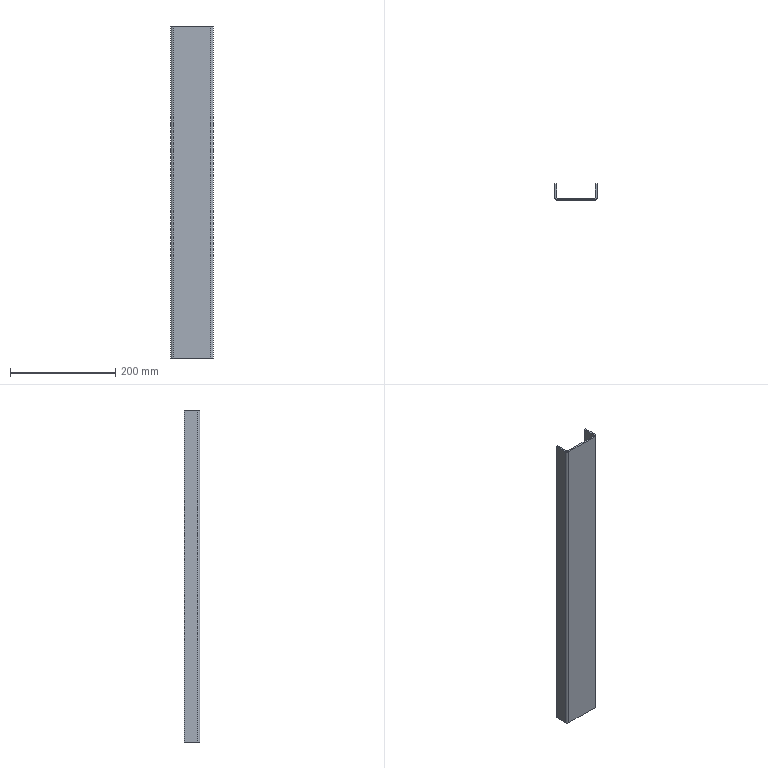Part | STEP file | 1 solid | 22 faces | box 80 x 30 x 630 mm | volume 248393 mm3 | plane 18 | cylinder 4 | commonest cylinder face diameters 3 x2 9 x2
STEP:
#1=CARTESIAN_POINT('',(0.,0.,0.));
#2=DIRECTION('',(0.,0.,1.));
#3=DIRECTION('',(1.,0.,0.));
#4=AXIS2_PLACEMENT_3D('',#1,#2,#3);
#5=CARTESIAN_POINT('',(35.5,-6.24,630.));
#6=VERTEX_POINT('',#5);
#7=CARTESIAN_POINT('',(35.5,-3.24,630.));
#8=VERTEX_POINT('',#7);
#9=CARTESIAN_POINT('',(35.5,-6.24,630.));
#10=DIRECTION('',(0.,1.,0.));
#11=VECTOR('',#10,1.);
#12=LINE('',#9,#11);
#13=CARTESIAN_POINT('',(35.5,-6.24,630.));
#14=DIRECTION('',(0.,0.,1.));
#15=DIRECTION('',(1.,0.,0.));
#16=AXIS2_PLACEMENT_3D('',#13,#14,#15);
#17=PLANE('',#16);
#18=CARTESIAN_POINT('',(0.,0.));
#19=DIRECTION('',(0.,1.));
#20=VECTOR('',#19,1.);
#21=LINE('',#18,#20);
#22=(GEOMETRIC_REPRESENTATION_CONTEXT(2)PARAMETRIC_REPRESENTATION_CONTEXT()REPRESENTATION_CONTEXT('',''));
#23=DEFINITIONAL_REPRESENTATION('',(#21),#22);
#24=PCURVE('',#17,#23);
#25=CARTESIAN_POINT('',(37.,-1.74,630.));
#26=DIRECTION('',(0.,0.,1.));
#27=DIRECTION('',(1.,0.,0.));
#28=AXIS2_PLACEMENT_3D('',#25,#26,#27);
#29=PLANE('',#28);
#30=CARTESIAN_POINT('',(-1.5,-4.5));
#31=DIRECTION('',(0.,1.));
#32=VECTOR('',#31,1.);
#33=LINE('',#30,#32);
#34=(GEOMETRIC_REPRESENTATION_CONTEXT(2)PARAMETRIC_REPRESENTATION_CONTEXT()REPRESENTATION_CONTEXT('',''));
#35=DEFINITIONAL_REPRESENTATION('',(#33),#34);
#36=PCURVE('',#29,#35);
#37=SURFACE_CURVE('',#12,(#24,#36),.PCURVE_S1.);
#38=EDGE_CURVE('',#6,#8,#37,.T.);
#39=ORIENTED_EDGE('',*,*,#38,.F.);
#40=CARTESIAN_POINT('',(40.,-1.74,630.));
#41=VERTEX_POINT('',#40);
#42=CARTESIAN_POINT('',(35.5,-1.74,630.));
#43=DIRECTION('',(0.,0.,-1.));
#44=DIRECTION('',(1.,0.,0.));
#45=AXIS2_PLACEMENT_3D('',#42,#43,#44);
#46=CIRCLE('',#45,4.5);
#47=CARTESIAN_POINT('',(4.5,4.5));
#48=CARTESIAN_POINT('',(4.5,-3.294));
#49=CARTESIAN_POINT('',(-2.25,0.6029));
#50=CARTESIAN_POINT('',(-9.,4.5));
#51=CARTESIAN_POINT('',(-2.25,8.397));
#52=CARTESIAN_POINT('',(4.5,12.294));
#53=CARTESIAN_POINT('',(4.5,4.5));
#54=(BOUNDED_CURVE()B_SPLINE_CURVE(2,(#47,#48,#49,#50,#51,#52,#53),.UNSPECIFIED.,.T.,.F.)B_SPLINE_CURVE_WITH_KNOTS((1,2,2,2,2,1),(-2.094,0.,2.094,4.189,6.283,8.378),.UNSPECIFIED.)CURVE()GEOMETRIC_REPRESENTATION_ITEM()RATIONAL_B_SPLINE_CURVE((1.,0.5,1.,0.5,1.,0.5,1.))REPRESENTATION_ITEM(''));
#55=(GEOMETRIC_REPRESENTATION_CONTEXT(2)PARAMETRIC_REPRESENTATION_CONTEXT()REPRESENTATION_CONTEXT('',''));
#56=DEFINITIONAL_REPRESENTATION('',(#54),#55);
#57=PCURVE('',#17,#56);
#58=CARTESIAN_POINT('',(35.5,-1.74,630.));
#59=DIRECTION('',(0.,0.,-1.));
#60=DIRECTION('',(-1.,0.,0.));
#61=AXIS2_PLACEMENT_3D('',#58,#59,#60);
#62=CYLINDRICAL_SURFACE('',#61,4.5);
#63=CARTESIAN_POINT('',(3.142,0.));
#64=DIRECTION('',(1.,0.));
#65=VECTOR('',#64,1.);
#66=LINE('',#63,#65);
#67=(GEOMETRIC_REPRESENTATION_CONTEXT(2)PARAMETRIC_REPRESENTATION_CONTEXT()REPRESENTATION_CONTEXT('',''));
#68=DEFINITIONAL_REPRESENTATION('',(#66),#67);
#69=PCURVE('',#62,#68);
#70=SURFACE_CURVE('',#46,(#57,#69),.PCURVE_S1.);
#71=EDGE_CURVE('',#41,#6,#70,.T.);
#72=ORIENTED_EDGE('',*,*,#71,.F.);
#73=CARTESIAN_POINT('',(37.,-1.74,630.));
#74=VERTEX_POINT('',#73);
#75=CARTESIAN_POINT('',(37.,-1.74,630.));
#76=DIRECTION('',(1.,0.,0.));
#77=VECTOR('',#76,1.);
#78=LINE('',#75,#77);
#79=CARTESIAN_POINT('',(1.5,4.5));
#80=DIRECTION('',(1.,0.));
#81=VECTOR('',#80,1.);
#82=LINE('',#79,#81);
#83=(GEOMETRIC_REPRESENTATION_CONTEXT(2)PARAMETRIC_REPRESENTATION_CONTEXT()REPRESENTATION_CONTEXT('',''));
#84=DEFINITIONAL_REPRESENTATION('',(#82),#83);
#85=PCURVE('',#17,#84);
#86=CARTESIAN_POINT('',(-35.5,-1.74,630.));
#87=DIRECTION('',(0.,0.,1.));
#88=DIRECTION('',(1.,0.,0.));
#89=AXIS2_PLACEMENT_3D('',#86,#87,#88);
#90=PLANE('',#89);
#91=CARTESIAN_POINT('',(72.5,0.));
#92=DIRECTION('',(1.,0.));
#93=VECTOR('',#92,1.);
#94=LINE('',#91,#93);
#95=(GEOMETRIC_REPRESENTATION_CONTEXT(2)PARAMETRIC_REPRESENTATION_CONTEXT()REPRESENTATION_CONTEXT('',''));
#96=DEFINITIONAL_REPRESENTATION('',(#94),#95);
#97=PCURVE('',#90,#96);
#98=SURFACE_CURVE('',#78,(#85,#97),.PCURVE_S1.);
#99=EDGE_CURVE('',#74,#41,#98,.T.);
#100=ORIENTED_EDGE('',*,*,#99,.F.);
#101=CARTESIAN_POINT('',(35.5,-1.74,630.));
#102=DIRECTION('',(0.,0.,-1.));
#103=DIRECTION('',(1.,0.,0.));
#104=AXIS2_PLACEMENT_3D('',#101,#102,#103);
#105=CIRCLE('',#104,1.5);
#106=CARTESIAN_POINT('',(1.5,4.5));
#107=CARTESIAN_POINT('',(1.5,1.902));
#108=CARTESIAN_POINT('',(-0.75,3.201));
#109=CARTESIAN_POINT('',(-3.,4.5));
#110=CARTESIAN_POINT('',(-0.75,5.799));
#111=CARTESIAN_POINT('',(1.5,7.098));
#112=CARTESIAN_POINT('',(1.5,4.5));
#113=(BOUNDED_CURVE()B_SPLINE_CURVE(2,(#106,#107,#108,#109,#110,#111,#112),.UNSPECIFIED.,.T.,.F.)B_SPLINE_CURVE_WITH_KNOTS((1,2,2,2,2,1),(-2.094,0.,2.094,4.189,6.283,8.378),.UNSPECIFIED.)CURVE()GEOMETRIC_REPRESENTATION_ITEM()RATIONAL_B_SPLINE_CURVE((1.,0.5,1.,0.5,1.,0.5,1.))REPRESENTATION_ITEM(''));
#114=(GEOMETRIC_REPRESENTATION_CONTEXT(2)PARAMETRIC_REPRESENTATION_CONTEXT()REPRESENTATION_CONTEXT('',''));
#115=DEFINITIONAL_REPRESENTATION('',(#113),#114);
#116=PCURVE('',#17,#115);
#117=CARTESIAN_POINT('',(35.5,-1.74,630.));
#118=DIRECTION('',(0.,0.,-1.));
#119=DIRECTION('',(-1.,0.,0.));
#120=AXIS2_PLACEMENT_3D('',#117,#118,#119);
#121=CYLINDRICAL_SURFACE('',#120,1.5);
#122=CARTESIAN_POINT('',(3.142,0.));
#123=DIRECTION('',(1.,0.));
#124=VECTOR('',#123,1.);
#125=LINE('',#122,#124);
#126=(GEOMETRIC_REPRESENTATION_CONTEXT(2)PARAMETRIC_REPRESENTATION_CONTEXT()REPRESENTATION_CONTEXT('',''));
#127=DEFINITIONAL_REPRESENTATION('',(#125),#126);
#128=PCURVE('',#121,#127);
#129=SURFACE_CURVE('',#105,(#116,#128),.PCURVE_S1.);
#130=EDGE_CURVE('',#74,#8,#129,.T.);
#131=ORIENTED_EDGE('',*,*,#130,.T.);
#132=EDGE_LOOP('',(#39,#72,#100,#131));
#133=FACE_BOUND('',#132,.T.);
#134=ADVANCED_FACE('',(#133),#17,.T.);
#135=CARTESIAN_POINT('',(-35.5,-6.24,630.));
#136=VERTEX_POINT('',#135);
#137=CARTESIAN_POINT('',(-40.,-6.24,630.));
#138=DIRECTION('',(-1.,0.,0.));
#139=VECTOR('',#138,1.);
#140=LINE('',#137,#139);
#141=CARTESIAN_POINT('',(-77.,-4.5));
#142=DIRECTION('',(-1.,0.));
#143=VECTOR('',#142,1.);
#144=LINE('',#141,#143);
#145=(GEOMETRIC_REPRESENTATION_CONTEXT(2)PARAMETRIC_REPRESENTATION_CONTEXT()REPRESENTATION_CONTEXT('',''));
#146=DEFINITIONAL_REPRESENTATION('',(#144),#145);
#147=PCURVE('',#29,#146);
#148=CARTESIAN_POINT('',(-40.,-6.24,630.));
#149=DIRECTION('',(0.,-1.,0.));
#150=DIRECTION('',(0.,0.,-1.));
#151=AXIS2_PLACEMENT_3D('',#148,#149,#150);
#152=PLANE('',#151);
#153=CARTESIAN_POINT('',(0.,0.));
#154=DIRECTION('',(0.,-1.));
#155=VECTOR('',#154,1.);
#156=LINE('',#153,#155);
#157=(GEOMETRIC_REPRESENTATION_CONTEXT(2)PARAMETRIC_REPRESENTATION_CONTEXT()REPRESENTATION_CONTEXT('',''));
#158=DEFINITIONAL_REPRESENTATION('',(#156),#157);
#159=PCURVE('',#152,#158);
#160=SURFACE_CURVE('',#140,(#147,#159),.PCURVE_S1.);
#161=EDGE_CURVE('',#6,#136,#160,.T.);
#162=ORIENTED_EDGE('',*,*,#161,.F.);
#163=ORIENTED_EDGE('',*,*,#38,.T.);
#164=CARTESIAN_POINT('',(-35.5,-3.24,630.));
#165=VERTEX_POINT('',#164);
#166=CARTESIAN_POINT('',(-40.,-3.24,630.));
#167=DIRECTION('',(-1.,0.,0.));
#168=VECTOR('',#167,1.);
#169=LINE('',#166,#168);
#170=CARTESIAN_POINT('',(-77.,-1.5));
#171=DIRECTION('',(-1.,0.));
#172=VECTOR('',#171,1.);
#173=LINE('',#170,#172);
#174=(GEOMETRIC_REPRESENTATION_CONTEXT(2)PARAMETRIC_REPRESENTATION_CONTEXT()REPRESENTATION_CONTEXT('',''));
#175=DEFINITIONAL_REPRESENTATION('',(#173),#174);
#176=PCURVE('',#29,#175);
#177=CARTESIAN_POINT('',(-40.,-3.24,630.));
#178=DIRECTION('',(0.,-1.,0.));
#179=DIRECTION('',(0.,0.,-1.));
#180=AXIS2_PLACEMENT_3D('',#177,#178,#179);
#181=PLANE('',#180);
#182=CARTESIAN_POINT('',(0.,0.));
#183=DIRECTION('',(0.,-1.));
#184=VECTOR('',#183,1.);
#185=LINE('',#182,#184);
#186=(GEOMETRIC_REPRESENTATION_CONTEXT(2)PARAMETRIC_REPRESENTATION_CONTEXT()REPRESENTATION_CONTEXT('',''));
#187=DEFINITIONAL_REPRESENTATION('',(#185),#186);
#188=PCURVE('',#181,#187);
#189=SURFACE_CURVE('',#169,(#176,#188),.PCURVE_S1.);
#190=EDGE_CURVE('',#8,#165,#189,.T.);
#191=ORIENTED_EDGE('',*,*,#190,.T.);
#192=CARTESIAN_POINT('',(-35.5,-3.24,630.));
#193=DIRECTION('',(0.,-1.,0.));
#194=VECTOR('',#193,1.);
#195=LINE('',#192,#194);
#196=CARTESIAN_POINT('',(-72.5,-1.5));
#197=DIRECTION('',(0.,-1.));
#198=VECTOR('',#197,1.);
#199=LINE('',#196,#198);
#200=(GEOMETRIC_REPRESENTATION_CONTEXT(2)PARAMETRIC_REPRESENTATION_CONTEXT()REPRESENTATION_CONTEXT('',''));
#201=DEFINITIONAL_REPRESENTATION('',(#199),#200);
#202=PCURVE('',#29,#201);
#203=CARTESIAN_POINT('',(-40.,-1.74,630.));
#204=DIRECTION('',(0.,0.,1.));
#205=DIRECTION('',(1.,0.,0.));
#206=AXIS2_PLACEMENT_3D('',#203,#204,#205);
#207=PLANE('',#206);
#208=CARTESIAN_POINT('',(4.5,-1.5));
#209=DIRECTION('',(0.,-1.));
#210=VECTOR('',#209,1.);
#211=LINE('',#208,#210);
#212=(GEOMETRIC_REPRESENTATION_CONTEXT(2)PARAMETRIC_REPRESENTATION_CONTEXT()REPRESENTATION_CONTEXT('',''));
#213=DEFINITIONAL_REPRESENTATION('',(#211),#212);
#214=PCURVE('',#207,#213);
#215=SURFACE_CURVE('',#195,(#202,#214),.PCURVE_S1.);
#216=EDGE_CURVE('',#165,#136,#215,.T.);
#217=ORIENTED_EDGE('',*,*,#216,.T.);
#218=EDGE_LOOP('',(#162,#163,#191,#217));
#219=FACE_BOUND('',#218,.T.);
#220=ADVANCED_FACE('',(#219),#29,.T.);
#221=CARTESIAN_POINT('',(40.,-1.74,0.));
#222=VERTEX_POINT('',#221);
#223=CARTESIAN_POINT('',(37.,-1.74,0.));
#224=VERTEX_POINT('',#223);
#225=CARTESIAN_POINT('',(40.,-1.74,0.));
#226=DIRECTION('',(-1.,0.,0.));
#227=VECTOR('',#226,1.);
#228=LINE('',#225,#227);
#229=CARTESIAN_POINT('',(40.,-1.74,0.));
#230=DIRECTION('',(0.,0.,-1.));
#231=DIRECTION('',(-1.,0.,0.));
#232=AXIS2_PLACEMENT_3D('',#229,#230,#231);
#233=PLANE('',#232);
#234=CARTESIAN_POINT('',(0.,0.));
#235=DIRECTION('',(1.,0.));
#236=VECTOR('',#235,1.);
#237=LINE('',#234,#236);
#238=(GEOMETRIC_REPRESENTATION_CONTEXT(2)PARAMETRIC_REPRESENTATION_CONTEXT()REPRESENTATION_CONTEXT('',''));
#239=DEFINITIONAL_REPRESENTATION('',(#237),#238);
#240=PCURVE('',#233,#239);
#241=CARTESIAN_POINT('',(35.5,-3.24,0.));
#242=DIRECTION('',(0.,0.,-1.));
#243=DIRECTION('',(-1.,0.,0.));
#244=AXIS2_PLACEMENT_3D('',#241,#242,#243);
#245=PLANE('',#244);
#246=CARTESIAN_POINT('',(-4.5,1.5));
#247=DIRECTION('',(1.,0.));
#248=VECTOR('',#247,1.);
#249=LINE('',#246,#248);
#250=(GEOMETRIC_REPRESENTATION_CONTEXT(2)PARAMETRIC_REPRESENTATION_CONTEXT()REPRESENTATION_CONTEXT('',''));
#251=DEFINITIONAL_REPRESENTATION('',(#249),#250);
#252=PCURVE('',#245,#251);
#253=SURFACE_CURVE('',#228,(#240,#252),.PCURVE_S1.);
#254=EDGE_CURVE('',#222,#224,#253,.T.);
#255=ORIENTED_EDGE('',*,*,#254,.F.);
#256=CARTESIAN_POINT('',(35.5,-6.24,0.));
#257=VERTEX_POINT('',#256);
#258=CARTESIAN_POINT('',(35.5,-1.74,0.));
#259=DIRECTION('',(0.,0.,-1.));
#260=DIRECTION('',(1.,0.,0.));
#261=AXIS2_PLACEMENT_3D('',#258,#259,#260);
#262=CIRCLE('',#261,4.5);
#263=CARTESIAN_POINT('',(4.5,0.));
#264=DIRECTION('',(-1.,0.));
#265=AXIS2_PLACEMENT_2D('',#263,#264);
#266=CIRCLE('',#265,4.5);
#267=(GEOMETRIC_REPRESENTATION_CONTEXT(2)PARAMETRIC_REPRESENTATION_CONTEXT()REPRESENTATION_CONTEXT('',''));
#268=DEFINITIONAL_REPRESENTATION('',(#266),#267);
#269=PCURVE('',#233,#268);
#270=CARTESIAN_POINT('',(3.142,630.));
#271=DIRECTION('',(1.,0.));
#272=VECTOR('',#271,1.);
#273=LINE('',#270,#272);
#274=(GEOMETRIC_REPRESENTATION_CONTEXT(2)PARAMETRIC_REPRESENTATION_CONTEXT()REPRESENTATION_CONTEXT('',''));
#275=DEFINITIONAL_REPRESENTATION('',(#273),#274);
#276=PCURVE('',#62,#275);
#277=SURFACE_CURVE('',#262,(#269,#276),.PCURVE_S1.);
#278=EDGE_CURVE('',#222,#257,#277,.T.);
#279=ORIENTED_EDGE('',*,*,#278,.T.);
#280=CARTESIAN_POINT('',(35.5,-3.24,0.));
#281=VERTEX_POINT('',#280);
#282=CARTESIAN_POINT('',(35.5,-3.24,0.));
#283=DIRECTION('',(0.,-1.,0.));
#284=VECTOR('',#283,1.);
#285=LINE('',#282,#284);
#286=CARTESIAN_POINT('',(4.5,-1.5));
#287=DIRECTION('',(0.,-1.));
#288=VECTOR('',#287,1.);
#289=LINE('',#286,#288);
#290=(GEOMETRIC_REPRESENTATION_CONTEXT(2)PARAMETRIC_REPRESENTATION_CONTEXT()REPRESENTATION_CONTEXT('',''));
#291=DEFINITIONAL_REPRESENTATION('',(#289),#290);
#292=PCURVE('',#233,#291);
#293=CARTESIAN_POINT('',(-37.,-1.74,0.));
#294=DIRECTION('',(0.,0.,-1.));
#295=DIRECTION('',(-1.,0.,0.));
#296=AXIS2_PLACEMENT_3D('',#293,#294,#295);
#297=PLANE('',#296);
#298=CARTESIAN_POINT('',(-72.5,-1.5));
#299=DIRECTION('',(0.,-1.));
#300=VECTOR('',#299,1.);
#301=LINE('',#298,#300);
#302=(GEOMETRIC_REPRESENTATION_CONTEXT(2)PARAMETRIC_REPRESENTATION_CONTEXT()REPRESENTATION_CONTEXT('',''));
#303=DEFINITIONAL_REPRESENTATION('',(#301),#302);
#304=PCURVE('',#297,#303);
#305=SURFACE_CURVE('',#285,(#292,#304),.PCURVE_S1.);
#306=EDGE_CURVE('',#281,#257,#305,.T.);
#307=ORIENTED_EDGE('',*,*,#306,.F.);
#308=CARTESIAN_POINT('',(35.5,-1.74,0.));
#309=DIRECTION('',(0.,0.,-1.));
#310=DIRECTION('',(1.,0.,0.));
#311=AXIS2_PLACEMENT_3D('',#308,#309,#310);
#312=CIRCLE('',#311,1.5);
#313=CARTESIAN_POINT('',(4.5,0.));
#314=DIRECTION('',(-1.,0.));
#315=AXIS2_PLACEMENT_2D('',#313,#314);
#316=CIRCLE('',#315,1.5);
#317=(GEOMETRIC_REPRESENTATION_CONTEXT(2)PARAMETRIC_REPRESENTATION_CONTEXT()REPRESENTATION_CONTEXT('',''));
#318=DEFINITIONAL_REPRESENTATION('',(#316),#317);
#319=PCURVE('',#233,#318);
#320=CARTESIAN_POINT('',(3.142,630.));
#321=DIRECTION('',(1.,0.));
#322=VECTOR('',#321,1.);
#323=LINE('',#320,#322);
#324=(GEOMETRIC_REPRESENTATION_CONTEXT(2)PARAMETRIC_REPRESENTATION_CONTEXT()REPRESENTATION_CONTEXT('',''));
#325=DEFINITIONAL_REPRESENTATION('',(#323),#324);
#326=PCURVE('',#121,#325);
#327=SURFACE_CURVE('',#312,(#319,#326),.PCURVE_S1.);
#328=EDGE_CURVE('',#224,#281,#327,.T.);
#329=ORIENTED_EDGE('',*,*,#328,.F.);
#330=EDGE_LOOP('',(#255,#279,#307,#329));
#331=FACE_BOUND('',#330,.T.);
#332=ADVANCED_FACE('',(#331),#233,.T.);
#333=CARTESIAN_POINT('',(40.,23.76,0.));
#334=VERTEX_POINT('',#333);
#335=CARTESIAN_POINT('',(40.,-6.24,0.));
#336=DIRECTION('',(0.,-1.,0.));
#337=VECTOR('',#336,1.);
#338=LINE('',#335,#337);
#339=CARTESIAN_POINT('',(-4.5,-3.));
#340=DIRECTION('',(0.,-1.));
#341=VECTOR('',#340,1.);
#342=LINE('',#339,#341);
#343=(GEOMETRIC_REPRESENTATION_CONTEXT(2)PARAMETRIC_REPRESENTATION_CONTEXT()REPRESENTATION_CONTEXT('',''));
#344=DEFINITIONAL_REPRESENTATION('',(#342),#343);
#345=PCURVE('',#245,#344);
#346=CARTESIAN_POINT('',(40.,-6.24,630.));
#347=DIRECTION('',(1.,0.,0.));
#348=DIRECTION('',(0.,0.,-1.));
#349=AXIS2_PLACEMENT_3D('',#346,#347,#348);
#350=PLANE('',#349);
#351=CARTESIAN_POINT('',(630.,0.));
#352=DIRECTION('',(0.,-1.));
#353=VECTOR('',#352,1.);
#354=LINE('',#351,#353);
#355=(GEOMETRIC_REPRESENTATION_CONTEXT(2)PARAMETRIC_REPRESENTATION_CONTEXT()REPRESENTATION_CONTEXT('',''));
#356=DEFINITIONAL_REPRESENTATION('',(#354),#355);
#357=PCURVE('',#350,#356);
#358=SURFACE_CURVE('',#338,(#345,#357),.PCURVE_S1.);
#359=EDGE_CURVE('',#334,#222,#358,.T.);
#360=ORIENTED_EDGE('',*,*,#359,.T.);
#361=ORIENTED_EDGE('',*,*,#254,.T.);
#362=CARTESIAN_POINT('',(37.,23.76,0.));
#363=VERTEX_POINT('',#362);
#364=CARTESIAN_POINT('',(37.,-6.24,0.));
#365=DIRECTION('',(0.,-1.,0.));
#366=VECTOR('',#365,1.);
#367=LINE('',#364,#366);
#368=CARTESIAN_POINT('',(-1.5,-3.));
#369=DIRECTION('',(0.,-1.));
#370=VECTOR('',#369,1.);
#371=LINE('',#368,#370);
#372=(GEOMETRIC_REPRESENTATION_CONTEXT(2)PARAMETRIC_REPRESENTATION_CONTEXT()REPRESENTATION_CONTEXT('',''));
#373=DEFINITIONAL_REPRESENTATION('',(#371),#372);
#374=PCURVE('',#245,#373);
#375=CARTESIAN_POINT('',(37.,-6.24,630.));
#376=DIRECTION('',(1.,0.,0.));
#377=DIRECTION('',(0.,0.,-1.));
#378=AXIS2_PLACEMENT_3D('',#375,#376,#377);
#379=PLANE('',#378);
#380=CARTESIAN_POINT('',(630.,0.));
#381=DIRECTION('',(0.,-1.));
#382=VECTOR('',#381,1.);
#383=LINE('',#380,#382);
#384=(GEOMETRIC_REPRESENTATION_CONTEXT(2)PARAMETRIC_REPRESENTATION_CONTEXT()REPRESENTATION_CONTEXT('',''));
#385=DEFINITIONAL_REPRESENTATION('',(#383),#384);
#386=PCURVE('',#379,#385);
#387=SURFACE_CURVE('',#367,(#374,#386),.PCURVE_S1.);
#388=EDGE_CURVE('',#363,#224,#387,.T.);
#389=ORIENTED_EDGE('',*,*,#388,.F.);
#390=CARTESIAN_POINT('',(37.,23.76,0.));
#391=DIRECTION('',(1.,0.,0.));
#392=VECTOR('',#391,1.);
#393=LINE('',#390,#392);
#394=CARTESIAN_POINT('',(-1.5,27.));
#395=DIRECTION('',(-1.,0.));
#396=VECTOR('',#395,1.);
#397=LINE('',#394,#396);
#398=(GEOMETRIC_REPRESENTATION_CONTEXT(2)PARAMETRIC_REPRESENTATION_CONTEXT()REPRESENTATION_CONTEXT('',''));
#399=DEFINITIONAL_REPRESENTATION('',(#397),#398);
#400=PCURVE('',#245,#399);
#401=CARTESIAN_POINT('',(37.,23.76,630.));
#402=DIRECTION('',(0.,1.,0.));
#403=DIRECTION('',(0.,0.,1.));
#404=AXIS2_PLACEMENT_3D('',#401,#402,#403);
#405=PLANE('',#404);
#406=CARTESIAN_POINT('',(-630.,0.));
#407=DIRECTION('',(0.,1.));
#408=VECTOR('',#407,1.);
#409=LINE('',#406,#408);
#410=(GEOMETRIC_REPRESENTATION_CONTEXT(2)PARAMETRIC_REPRESENTATION_CONTEXT()REPRESENTATION_CONTEXT('',''));
#411=DEFINITIONAL_REPRESENTATION('',(#409),#410);
#412=PCURVE('',#405,#411);
#413=SURFACE_CURVE('',#393,(#400,#412),.PCURVE_S1.);
#414=EDGE_CURVE('',#363,#334,#413,.T.);
#415=ORIENTED_EDGE('',*,*,#414,.T.);
#416=EDGE_LOOP('',(#360,#361,#389,#415));
#417=FACE_BOUND('',#416,.T.);
#418=ADVANCED_FACE('',(#417),#245,.T.);
#419=CARTESIAN_POINT('',(-40.,-1.74,630.));
#420=VERTEX_POINT('',#419);
#421=CARTESIAN_POINT('',(-37.,-1.74,630.));
#422=VERTEX_POINT('',#421);
#423=CARTESIAN_POINT('',(-40.,-1.74,630.));
#424=DIRECTION('',(1.,0.,0.));
#425=VECTOR('',#424,1.);
#426=LINE('',#423,#425);
#427=CARTESIAN_POINT('',(0.,0.));
#428=DIRECTION('',(1.,0.));
#429=VECTOR('',#428,1.);
#430=LINE('',#427,#429);
#431=(GEOMETRIC_REPRESENTATION_CONTEXT(2)PARAMETRIC_REPRESENTATION_CONTEXT()REPRESENTATION_CONTEXT('',''));
#432=DEFINITIONAL_REPRESENTATION('',(#430),#431);
#433=PCURVE('',#207,#432);
#434=CARTESIAN_POINT('',(-35.5,-3.24,630.));
#435=DIRECTION('',(0.,0.,1.));
#436=DIRECTION('',(1.,0.,0.));
#437=AXIS2_PLACEMENT_3D('',#434,#435,#436);
#438=PLANE('',#437);
#439=CARTESIAN_POINT('',(-4.5,1.5));
#440=DIRECTION('',(1.,0.));
#441=VECTOR('',#440,1.);
#442=LINE('',#439,#441);
#443=(GEOMETRIC_REPRESENTATION_CONTEXT(2)PARAMETRIC_REPRESENTATION_CONTEXT()REPRESENTATION_CONTEXT('',''));
#444=DEFINITIONAL_REPRESENTATION('',(#442),#443);
#445=PCURVE('',#438,#444);
#446=SURFACE_CURVE('',#426,(#433,#445),.PCURVE_S1.);
#447=EDGE_CURVE('',#420,#422,#446,.T.);
#448=ORIENTED_EDGE('',*,*,#447,.F.);
#449=CARTESIAN_POINT('',(-35.5,-1.74,630.));
#450=DIRECTION('',(0.,0.,-1.));
#451=DIRECTION('',(1.,0.,0.));
#452=AXIS2_PLACEMENT_3D('',#449,#450,#451);
#453=CIRCLE('',#452,4.5);
#454=CARTESIAN_POINT('',(9.,0.));
#455=CARTESIAN_POINT('',(9.,-7.794));
#456=CARTESIAN_POINT('',(2.25,-3.897));
#457=CARTESIAN_POINT('',(-4.5,0.));
#458=CARTESIAN_POINT('',(2.25,3.897));
#459=CARTESIAN_POINT('',(9.,7.794));
#460=CARTESIAN_POINT('',(9.,0.));
#461=(BOUNDED_CURVE()B_SPLINE_CURVE(2,(#454,#455,#456,#457,#458,#459,#460),.UNSPECIFIED.,.T.,.F.)B_SPLINE_CURVE_WITH_KNOTS((1,2,2,2,2,1),(-2.094,0.,2.094,4.189,6.283,8.378),.UNSPECIFIED.)CURVE()GEOMETRIC_REPRESENTATION_ITEM()RATIONAL_B_SPLINE_CURVE((1.,0.5,1.,0.5,1.,0.5,1.))REPRESENTATION_ITEM(''));
#462=(GEOMETRIC_REPRESENTATION_CONTEXT(2)PARAMETRIC_REPRESENTATION_CONTEXT()REPRESENTATION_CONTEXT('',''));
#463=DEFINITIONAL_REPRESENTATION('',(#461),#462);
#464=PCURVE('',#207,#463);
#465=CARTESIAN_POINT('',(-35.5,-1.74,630.));
#466=DIRECTION('',(0.,0.,-1.));
#467=DIRECTION('',(-1.,0.,0.));
#468=AXIS2_PLACEMENT_3D('',#465,#466,#467);
#469=CYLINDRICAL_SURFACE('',#468,4.5);
#470=CARTESIAN_POINT('',(3.142,0.));
#471=DIRECTION('',(1.,0.));
#472=VECTOR('',#471,1.);
#473=LINE('',#470,#472);
#474=(GEOMETRIC_REPRESENTATION_CONTEXT(2)PARAMETRIC_REPRESENTATION_CONTEXT()REPRESENTATION_CONTEXT('',''));
#475=DEFINITIONAL_REPRESENTATION('',(#473),#474);
#476=PCURVE('',#469,#475);
#477=SURFACE_CURVE('',#453,(#464,#476),.PCURVE_S1.);
#478=EDGE_CURVE('',#136,#420,#477,.T.);
#479=ORIENTED_EDGE('',*,*,#478,.F.);
#480=ORIENTED_EDGE('',*,*,#216,.F.);
#481=CARTESIAN_POINT('',(-35.5,-1.74,630.));
#482=DIRECTION('',(0.,0.,-1.));
#483=DIRECTION('',(1.,0.,0.));
#484=AXIS2_PLACEMENT_3D('',#481,#482,#483);
#485=CIRCLE('',#484,1.5);
#486=CARTESIAN_POINT('',(6.,0.));
#487=CARTESIAN_POINT('',(6.,-2.598));
#488=CARTESIAN_POINT('',(3.75,-1.299));
#489=CARTESIAN_POINT('',(1.5,0.));
#490=CARTESIAN_POINT('',(3.75,1.299));
#491=CARTESIAN_POINT('',(6.,2.598));
#492=CARTESIAN_POINT('',(6.,0.));
#493=(BOUNDED_CURVE()B_SPLINE_CURVE(2,(#486,#487,#488,#489,#490,#491,#492),.UNSPECIFIED.,.T.,.F.)B_SPLINE_CURVE_WITH_KNOTS((1,2,2,2,2,1),(-2.094,0.,2.094,4.189,6.283,8.378),.UNSPECIFIED.)CURVE()GEOMETRIC_REPRESENTATION_ITEM()RATIONAL_B_SPLINE_CURVE((1.,0.5,1.,0.5,1.,0.5,1.))REPRESENTATION_ITEM(''));
#494=(GEOMETRIC_REPRESENTATION_CONTEXT(2)PARAMETRIC_REPRESENTATION_CONTEXT()REPRESENTATION_CONTEXT('',''));
#495=DEFINITIONAL_REPRESENTATION('',(#493),#494);
#496=PCURVE('',#207,#495);
#497=CARTESIAN_POINT('',(-35.5,-1.74,630.));
#498=DIRECTION('',(0.,0.,-1.));
#499=DIRECTION('',(-1.,0.,0.));
#500=AXIS2_PLACEMENT_3D('',#497,#498,#499);
#501=CYLINDRICAL_SURFACE('',#500,1.5);
#502=CARTESIAN_POINT('',(3.142,0.));
#503=DIRECTION('',(1.,0.));
#504=VECTOR('',#503,1.);
#505=LINE('',#502,#504);
#506=(GEOMETRIC_REPRESENTATION_CONTEXT(2)PARAMETRIC_REPRESENTATION_CONTEXT()REPRESENTATION_CONTEXT('',''));
#507=DEFINITIONAL_REPRESENTATION('',(#505),#506);
#508=PCURVE('',#501,#507);
#509=SURFACE_CURVE('',#485,(#496,#508),.PCURVE_S1.);
#510=EDGE_CURVE('',#165,#422,#509,.T.);
#511=ORIENTED_EDGE('',*,*,#510,.T.);
#512=EDGE_LOOP('',(#448,#479,#480,#511));
#513=FACE_BOUND('',#512,.T.);
#514=ADVANCED_FACE('',(#513),#207,.T.);
#515=CARTESIAN_POINT('',(-40.,23.76,630.));
#516=VERTEX_POINT('',#515);
#517=CARTESIAN_POINT('',(-40.,-6.24,630.));
#518=DIRECTION('',(0.,1.,0.));
#519=VECTOR('',#518,1.);
#520=LINE('',#517,#519);
#521=CARTESIAN_POINT('',(-4.5,-3.));
#522=DIRECTION('',(0.,1.));
#523=VECTOR('',#522,1.);
#524=LINE('',#521,#523);
#525=(GEOMETRIC_REPRESENTATION_CONTEXT(2)PARAMETRIC_REPRESENTATION_CONTEXT()REPRESENTATION_CONTEXT('',''));
#526=DEFINITIONAL_REPRESENTATION('',(#524),#525);
#527=PCURVE('',#438,#526);
#528=CARTESIAN_POINT('',(-40.,-6.24,630.));
#529=DIRECTION('',(-1.,0.,0.));
#530=DIRECTION('',(0.,0.,1.));
#531=AXIS2_PLACEMENT_3D('',#528,#529,#530);
#532=PLANE('',#531);
#533=CARTESIAN_POINT('',(0.,0.));
#534=DIRECTION('',(0.,1.));
#535=VECTOR('',#534,1.);
#536=LINE('',#533,#535);
#537=(GEOMETRIC_REPRESENTATION_CONTEXT(2)PARAMETRIC_REPRESENTATION_CONTEXT()REPRESENTATION_CONTEXT('',''));
#538=DEFINITIONAL_REPRESENTATION('',(#536),#537);
#539=PCURVE('',#532,#538);
#540=SURFACE_CURVE('',#520,(#527,#539),.PCURVE_S1.);
#541=EDGE_CURVE('',#420,#516,#540,.T.);
#542=ORIENTED_EDGE('',*,*,#541,.F.);
#543=ORIENTED_EDGE('',*,*,#447,.T.);
#544=CARTESIAN_POINT('',(-37.,23.76,630.));
#545=VERTEX_POINT('',#544);
#546=CARTESIAN_POINT('',(-37.,-6.24,630.));
#547=DIRECTION('',(0.,1.,0.));
#548=VECTOR('',#547,1.);
#549=LINE('',#546,#548);
#550=CARTESIAN_POINT('',(-1.5,-3.));
#551=DIRECTION('',(0.,1.));
#552=VECTOR('',#551,1.);
#553=LINE('',#550,#552);
#554=(GEOMETRIC_REPRESENTATION_CONTEXT(2)PARAMETRIC_REPRESENTATION_CONTEXT()REPRESENTATION_CONTEXT('',''));
#555=DEFINITIONAL_REPRESENTATION('',(#553),#554);
#556=PCURVE('',#438,#555);
#557=CARTESIAN_POINT('',(-37.,-6.24,630.));
#558=DIRECTION('',(-1.,0.,0.));
#559=DIRECTION('',(0.,0.,1.));
#560=AXIS2_PLACEMENT_3D('',#557,#558,#559);
#561=PLANE('',#560);
#562=CARTESIAN_POINT('',(0.,0.));
#563=DIRECTION('',(0.,1.));
#564=VECTOR('',#563,1.);
#565=LINE('',#562,#564);
#566=(GEOMETRIC_REPRESENTATION_CONTEXT(2)PARAMETRIC_REPRESENTATION_CONTEXT()REPRESENTATION_CONTEXT('',''));
#567=DEFINITIONAL_REPRESENTATION('',(#565),#566);
#568=PCURVE('',#561,#567);
#569=SURFACE_CURVE('',#549,(#556,#568),.PCURVE_S1.);
#570=EDGE_CURVE('',#422,#545,#569,.T.);
#571=ORIENTED_EDGE('',*,*,#570,.T.);
#572=CARTESIAN_POINT('',(-40.,23.76,630.));
#573=DIRECTION('',(1.,0.,0.));
#574=VECTOR('',#573,1.);
#575=LINE('',#572,#574);
#576=CARTESIAN_POINT('',(-4.5,27.));
#577=DIRECTION('',(1.,0.));
#578=VECTOR('',#577,1.);
#579=LINE('',#576,#578);
#580=(GEOMETRIC_REPRESENTATION_CONTEXT(2)PARAMETRIC_REPRESENTATION_CONTEXT()REPRESENTATION_CONTEXT('',''));
#581=DEFINITIONAL_REPRESENTATION('',(#579),#580);
#582=PCURVE('',#438,#581);
#583=CARTESIAN_POINT('',(-40.,23.76,630.));
#584=DIRECTION('',(0.,1.,0.));
#585=DIRECTION('',(0.,0.,1.));
#586=AXIS2_PLACEMENT_3D('',#583,#584,#585);
#587=PLANE('',#586);
#588=CARTESIAN_POINT('',(0.,0.));
#589=DIRECTION('',(0.,1.));
#590=VECTOR('',#589,1.);
#591=LINE('',#588,#590);
#592=(GEOMETRIC_REPRESENTATION_CONTEXT(2)PARAMETRIC_REPRESENTATION_CONTEXT()REPRESENTATION_CONTEXT('',''));
#593=DEFINITIONAL_REPRESENTATION('',(#591),#592);
#594=PCURVE('',#587,#593);
#595=SURFACE_CURVE('',#575,(#582,#594),.PCURVE_S1.);
#596=EDGE_CURVE('',#516,#545,#595,.T.);
#597=ORIENTED_EDGE('',*,*,#596,.F.);
#598=EDGE_LOOP('',(#542,#543,#571,#597));
#599=FACE_BOUND('',#598,.T.);
#600=ADVANCED_FACE('',(#599),#438,.T.);
#601=CARTESIAN_POINT('',(-35.5,-6.24,0.));
#602=VERTEX_POINT('',#601);
#603=CARTESIAN_POINT('',(-35.5,-3.24,0.));
#604=VERTEX_POINT('',#603);
#605=CARTESIAN_POINT('',(-35.5,-6.24,0.));
#606=DIRECTION('',(0.,1.,0.));
#607=VECTOR('',#606,1.);
#608=LINE('',#605,#607);
#609=CARTESIAN_POINT('',(-35.5,-6.24,0.));
#610=DIRECTION('',(0.,0.,-1.));
#611=DIRECTION('',(-1.,0.,0.));
#612=AXIS2_PLACEMENT_3D('',#609,#610,#611);
#613=PLANE('',#612);
#614=CARTESIAN_POINT('',(0.,0.));
#615=DIRECTION('',(0.,1.));
#616=VECTOR('',#615,1.);
#617=LINE('',#614,#616);
#618=(GEOMETRIC_REPRESENTATION_CONTEXT(2)PARAMETRIC_REPRESENTATION_CONTEXT()REPRESENTATION_CONTEXT('',''));
#619=DEFINITIONAL_REPRESENTATION('',(#617),#618);
#620=PCURVE('',#613,#619);
#621=CARTESIAN_POINT('',(-1.5,-4.5));
#622=DIRECTION('',(0.,1.));
#623=VECTOR('',#622,1.);
#624=LINE('',#621,#623);
#625=(GEOMETRIC_REPRESENTATION_CONTEXT(2)PARAMETRIC_REPRESENTATION_CONTEXT()REPRESENTATION_CONTEXT('',''));
#626=DEFINITIONAL_REPRESENTATION('',(#624),#625);
#627=PCURVE('',#297,#626);
#628=SURFACE_CURVE('',#608,(#620,#627),.PCURVE_S1.);
#629=EDGE_CURVE('',#602,#604,#628,.T.);
#630=ORIENTED_EDGE('',*,*,#629,.F.);
#631=CARTESIAN_POINT('',(-40.,-1.74,0.));
#632=VERTEX_POINT('',#631);
#633=CARTESIAN_POINT('',(-35.5,-1.74,0.));
#634=DIRECTION('',(0.,0.,-1.));
#635=DIRECTION('',(1.,0.,0.));
#636=AXIS2_PLACEMENT_3D('',#633,#634,#635);
#637=CIRCLE('',#636,4.5);
#638=CARTESIAN_POINT('',(0.,4.5));
#639=DIRECTION('',(-1.,0.));
#640=AXIS2_PLACEMENT_2D('',#638,#639);
#641=CIRCLE('',#640,4.5);
#642=(GEOMETRIC_REPRESENTATION_CONTEXT(2)PARAMETRIC_REPRESENTATION_CONTEXT()REPRESENTATION_CONTEXT('',''));
#643=DEFINITIONAL_REPRESENTATION('',(#641),#642);
#644=PCURVE('',#613,#643);
#645=CARTESIAN_POINT('',(3.142,630.));
#646=DIRECTION('',(1.,0.));
#647=VECTOR('',#646,1.);
#648=LINE('',#645,#647);
#649=(GEOMETRIC_REPRESENTATION_CONTEXT(2)PARAMETRIC_REPRESENTATION_CONTEXT()REPRESENTATION_CONTEXT('',''));
#650=DEFINITIONAL_REPRESENTATION('',(#648),#649);
#651=PCURVE('',#469,#650);
#652=SURFACE_CURVE('',#637,(#644,#651),.PCURVE_S1.);
#653=EDGE_CURVE('',#602,#632,#652,.T.);
#654=ORIENTED_EDGE('',*,*,#653,.T.);
#655=CARTESIAN_POINT('',(-37.,-1.74,0.));
#656=VERTEX_POINT('',#655);
#657=CARTESIAN_POINT('',(-37.,-1.74,0.));
#658=DIRECTION('',(-1.,0.,0.));
#659=VECTOR('',#658,1.);
#660=LINE('',#657,#659);
#661=CARTESIAN_POINT('',(1.5,4.5));
#662=DIRECTION('',(1.,0.));
#663=VECTOR('',#662,1.);
#664=LINE('',#661,#663);
#665=(GEOMETRIC_REPRESENTATION_CONTEXT(2)PARAMETRIC_REPRESENTATION_CONTEXT()REPRESENTATION_CONTEXT('',''));
#666=DEFINITIONAL_REPRESENTATION('',(#664),#665);
#667=PCURVE('',#613,#666);
#668=CARTESIAN_POINT('',(-35.5,-1.74,0.));
#669=DIRECTION('',(0.,0.,1.));
#670=DIRECTION('',(1.,0.,0.));
#671=AXIS2_PLACEMENT_3D('',#668,#669,#670);
#672=PLANE('',#671);
#673=CARTESIAN_POINT('',(-1.5,0.));
#674=DIRECTION('',(-1.,0.));
#675=VECTOR('',#674,1.);
#676=LINE('',#673,#675);
#677=(GEOMETRIC_REPRESENTATION_CONTEXT(2)PARAMETRIC_REPRESENTATION_CONTEXT()REPRESENTATION_CONTEXT('',''));
#678=DEFINITIONAL_REPRESENTATION('',(#676),#677);
#679=PCURVE('',#672,#678);
#680=SURFACE_CURVE('',#660,(#667,#679),.PCURVE_S1.);
#681=EDGE_CURVE('',#656,#632,#680,.T.);
#682=ORIENTED_EDGE('',*,*,#681,.F.);
#683=CARTESIAN_POINT('',(-35.5,-1.74,0.));
#684=DIRECTION('',(0.,0.,-1.));
#685=DIRECTION('',(1.,0.,0.));
#686=AXIS2_PLACEMENT_3D('',#683,#684,#685);
#687=CIRCLE('',#686,1.5);
#688=CARTESIAN_POINT('',(0.,4.5));
#689=DIRECTION('',(-1.,0.));
#690=AXIS2_PLACEMENT_2D('',#688,#689);
#691=CIRCLE('',#690,1.5);
#692=(GEOMETRIC_REPRESENTATION_CONTEXT(2)PARAMETRIC_REPRESENTATION_CONTEXT()REPRESENTATION_CONTEXT('',''));
#693=DEFINITIONAL_REPRESENTATION('',(#691),#692);
#694=PCURVE('',#613,#693);
#695=CARTESIAN_POINT('',(3.142,630.));
#696=DIRECTION('',(1.,0.));
#697=VECTOR('',#696,1.);
#698=LINE('',#695,#697);
#699=(GEOMETRIC_REPRESENTATION_CONTEXT(2)PARAMETRIC_REPRESENTATION_CONTEXT()REPRESENTATION_CONTEXT('',''));
#700=DEFINITIONAL_REPRESENTATION('',(#698),#699);
#701=PCURVE('',#501,#700);
#702=SURFACE_CURVE('',#687,(#694,#701),.PCURVE_S1.);
#703=EDGE_CURVE('',#604,#656,#702,.T.);
#704=ORIENTED_EDGE('',*,*,#703,.F.);
#705=EDGE_LOOP('',(#630,#654,#682,#704));
#706=FACE_BOUND('',#705,.T.);
#707=ADVANCED_FACE('',(#706),#613,.T.);
#708=CARTESIAN_POINT('',(-40.,-6.24,0.));
#709=DIRECTION('',(-1.,0.,0.));
#710=VECTOR('',#709,1.);
#711=LINE('',#708,#710);
#712=CARTESIAN_POINT('',(3.,-4.5));
#713=DIRECTION('',(1.,0.));
#714=VECTOR('',#713,1.);
#715=LINE('',#712,#714);
#716=(GEOMETRIC_REPRESENTATION_CONTEXT(2)PARAMETRIC_REPRESENTATION_CONTEXT()REPRESENTATION_CONTEXT('',''));
#717=DEFINITIONAL_REPRESENTATION('',(#715),#716);
#718=PCURVE('',#297,#717);
#719=CARTESIAN_POINT('',(630.,0.));
#720=DIRECTION('',(0.,-1.));
#721=VECTOR('',#720,1.);
#722=LINE('',#719,#721);
#723=(GEOMETRIC_REPRESENTATION_CONTEXT(2)PARAMETRIC_REPRESENTATION_CONTEXT()REPRESENTATION_CONTEXT('',''));
#724=DEFINITIONAL_REPRESENTATION('',(#722),#723);
#725=PCURVE('',#152,#724);
#726=SURFACE_CURVE('',#711,(#718,#725),.PCURVE_S1.);
#727=EDGE_CURVE('',#257,#602,#726,.T.);
#728=ORIENTED_EDGE('',*,*,#727,.T.);
#729=ORIENTED_EDGE('',*,*,#629,.T.);
#730=CARTESIAN_POINT('',(-40.,-3.24,0.));
#731=DIRECTION('',(-1.,0.,0.));
#732=VECTOR('',#731,1.);
#733=LINE('',#730,#732);
#734=CARTESIAN_POINT('',(3.,-1.5));
#735=DIRECTION('',(1.,0.));
#736=VECTOR('',#735,1.);
#737=LINE('',#734,#736);
#738=(GEOMETRIC_REPRESENTATION_CONTEXT(2)PARAMETRIC_REPRESENTATION_CONTEXT()REPRESENTATION_CONTEXT('',''));
#739=DEFINITIONAL_REPRESENTATION('',(#737),#738);
#740=PCURVE('',#297,#739);
#741=CARTESIAN_POINT('',(630.,0.));
#742=DIRECTION('',(0.,-1.));
#743=VECTOR('',#742,1.);
#744=LINE('',#741,#743);
#745=(GEOMETRIC_REPRESENTATION_CONTEXT(2)PARAMETRIC_REPRESENTATION_CONTEXT()REPRESENTATION_CONTEXT('',''));
#746=DEFINITIONAL_REPRESENTATION('',(#744),#745);
#747=PCURVE('',#181,#746);
#748=SURFACE_CURVE('',#733,(#740,#747),.PCURVE_S1.);
#749=EDGE_CURVE('',#281,#604,#748,.T.);
#750=ORIENTED_EDGE('',*,*,#749,.F.);
#751=ORIENTED_EDGE('',*,*,#306,.T.);
#752=EDGE_LOOP('',(#728,#729,#750,#751));
#753=FACE_BOUND('',#752,.T.);
#754=ADVANCED_FACE('',(#753),#297,.T.);
#755=CARTESIAN_POINT('',(-37.,23.76,0.));
#756=VERTEX_POINT('',#755);
#757=CARTESIAN_POINT('',(-37.,-6.24,0.));
#758=DIRECTION('',(0.,1.,0.));
#759=VECTOR('',#758,1.);
#760=LINE('',#757,#759);
#761=CARTESIAN_POINT('',(-630.,0.));
#762=DIRECTION('',(0.,1.));
#763=VECTOR('',#762,1.);
#764=LINE('',#761,#763);
#765=(GEOMETRIC_REPRESENTATION_CONTEXT(2)PARAMETRIC_REPRESENTATION_CONTEXT()REPRESENTATION_CONTEXT('',''));
#766=DEFINITIONAL_REPRESENTATION('',(#764),#765);
#767=PCURVE('',#561,#766);
#768=CARTESIAN_POINT('',(-1.5,-4.5));
#769=DIRECTION('',(0.,1.));
#770=VECTOR('',#769,1.);
#771=LINE('',#768,#770);
#772=(GEOMETRIC_REPRESENTATION_CONTEXT(2)PARAMETRIC_REPRESENTATION_CONTEXT()REPRESENTATION_CONTEXT('',''));
#773=DEFINITIONAL_REPRESENTATION('',(#771),#772);
#774=PCURVE('',#672,#773);
#775=SURFACE_CURVE('',#760,(#767,#774),.PCURVE_S1.);
#776=EDGE_CURVE('',#656,#756,#775,.T.);
#777=ORIENTED_EDGE('',*,*,#776,.T.);
#778=CARTESIAN_POINT('',(-37.,23.76,630.));
#779=DIRECTION('',(0.,0.,-1.));
#780=VECTOR('',#779,1.);
#781=LINE('',#778,#780);
#782=CARTESIAN_POINT('',(0.,30.));
#783=DIRECTION('',(-1.,0.));
#784=VECTOR('',#783,1.);
#785=LINE('',#782,#784);
#786=(GEOMETRIC_REPRESENTATION_CONTEXT(2)PARAMETRIC_REPRESENTATION_CONTEXT()REPRESENTATION_CONTEXT('',''));
#787=DEFINITIONAL_REPRESENTATION('',(#785),#786);
#788=PCURVE('',#561,#787);
#789=CARTESIAN_POINT('',(0.,3.));
#790=DIRECTION('',(-1.,0.));
#791=VECTOR('',#790,1.);
#792=LINE('',#789,#791);
#793=(GEOMETRIC_REPRESENTATION_CONTEXT(2)PARAMETRIC_REPRESENTATION_CONTEXT()REPRESENTATION_CONTEXT('',''));
#794=DEFINITIONAL_REPRESENTATION('',(#792),#793);
#795=PCURVE('',#587,#794);
#796=SURFACE_CURVE('',#781,(#788,#795),.PCURVE_S1.);
#797=EDGE_CURVE('',#545,#756,#796,.T.);
#798=ORIENTED_EDGE('',*,*,#797,.F.);
#799=ORIENTED_EDGE('',*,*,#570,.F.);
#800=CARTESIAN_POINT('',(-37.,-1.74,630.));
#801=DIRECTION('',(0.,0.,-1.));
#802=VECTOR('',#801,1.);
#803=LINE('',#800,#802);
#804=CARTESIAN_POINT('',(0.,4.5));
#805=DIRECTION('',(-1.,0.));
#806=VECTOR('',#805,1.);
#807=LINE('',#804,#806);
#808=(GEOMETRIC_REPRESENTATION_CONTEXT(2)PARAMETRIC_REPRESENTATION_CONTEXT()REPRESENTATION_CONTEXT('',''));
#809=DEFINITIONAL_REPRESENTATION('',(#807),#808);
#810=PCURVE('',#561,#809);
#811=CARTESIAN_POINT('',(6.283,0.));
#812=DIRECTION('',(0.,1.));
#813=VECTOR('',#812,1.);
#814=LINE('',#811,#813);
#815=(GEOMETRIC_REPRESENTATION_CONTEXT(2)PARAMETRIC_REPRESENTATION_CONTEXT()REPRESENTATION_CONTEXT('',''));
#816=DEFINITIONAL_REPRESENTATION('',(#814),#815);
#817=PCURVE('',#501,#816);
#818=SURFACE_CURVE('',#803,(#810,#817),.PCURVE_S1.);
#819=EDGE_CURVE('',#422,#656,#818,.T.);
#820=ORIENTED_EDGE('',*,*,#819,.T.);
#821=EDGE_LOOP('',(#777,#798,#799,#820));
#822=FACE_BOUND('',#821,.T.);
#823=ADVANCED_FACE('',(#822),#561,.F.);
#824=CARTESIAN_POINT('',(-40.,23.76,0.));
#825=VERTEX_POINT('',#824);
#826=CARTESIAN_POINT('',(-40.,23.76,0.));
#827=DIRECTION('',(1.,0.,0.));
#828=VECTOR('',#827,1.);
#829=LINE('',#826,#828);
#830=CARTESIAN_POINT('',(-630.,0.));
#831=DIRECTION('',(0.,1.));
#832=VECTOR('',#831,1.);
#833=LINE('',#830,#832);
#834=(GEOMETRIC_REPRESENTATION_CONTEXT(2)PARAMETRIC_REPRESENTATION_CONTEXT()REPRESENTATION_CONTEXT('',''));
#835=DEFINITIONAL_REPRESENTATION('',(#833),#834);
#836=PCURVE('',#587,#835);
#837=CARTESIAN_POINT('',(-4.5,25.5));
#838=DIRECTION('',(1.,0.));
#839=VECTOR('',#838,1.);
#840=LINE('',#837,#839);
#841=(GEOMETRIC_REPRESENTATION_CONTEXT(2)PARAMETRIC_REPRESENTATION_CONTEXT()REPRESENTATION_CONTEXT('',''));
#842=DEFINITIONAL_REPRESENTATION('',(#840),#841);
#843=PCURVE('',#672,#842);
#844=SURFACE_CURVE('',#829,(#836,#843),.PCURVE_S1.);
#845=EDGE_CURVE('',#825,#756,#844,.T.);
#846=ORIENTED_EDGE('',*,*,#845,.F.);
#847=CARTESIAN_POINT('',(-40.,23.76,630.));
#848=DIRECTION('',(0.,0.,-1.));
#849=VECTOR('',#848,1.);
#850=LINE('',#847,#849);
#851=CARTESIAN_POINT('',(0.,0.));
#852=DIRECTION('',(-1.,0.));
#853=VECTOR('',#852,1.);
#854=LINE('',#851,#853);
#855=(GEOMETRIC_REPRESENTATION_CONTEXT(2)PARAMETRIC_REPRESENTATION_CONTEXT()REPRESENTATION_CONTEXT('',''));
#856=DEFINITIONAL_REPRESENTATION('',(#854),#855);
#857=PCURVE('',#587,#856);
#858=CARTESIAN_POINT('',(0.,30.));
#859=DIRECTION('',(-1.,0.));
#860=VECTOR('',#859,1.);
#861=LINE('',#858,#860);
#862=(GEOMETRIC_REPRESENTATION_CONTEXT(2)PARAMETRIC_REPRESENTATION_CONTEXT()REPRESENTATION_CONTEXT('',''));
#863=DEFINITIONAL_REPRESENTATION('',(#861),#862);
#864=PCURVE('',#532,#863);
#865=SURFACE_CURVE('',#850,(#857,#864),.PCURVE_S1.);
#866=EDGE_CURVE('',#516,#825,#865,.T.);
#867=ORIENTED_EDGE('',*,*,#866,.F.);
#868=ORIENTED_EDGE('',*,*,#596,.T.);
#869=ORIENTED_EDGE('',*,*,#797,.T.);
#870=EDGE_LOOP('',(#846,#867,#868,#869));
#871=FACE_BOUND('',#870,.T.);
#872=ADVANCED_FACE('',(#871),#587,.T.);
#873=CARTESIAN_POINT('',(-40.,-6.24,0.));
#874=DIRECTION('',(0.,1.,0.));
#875=VECTOR('',#874,1.);
#876=LINE('',#873,#875);
#877=CARTESIAN_POINT('',(-630.,0.));
#878=DIRECTION('',(0.,1.));
#879=VECTOR('',#878,1.);
#880=LINE('',#877,#879);
#881=(GEOMETRIC_REPRESENTATION_CONTEXT(2)PARAMETRIC_REPRESENTATION_CONTEXT()REPRESENTATION_CONTEXT('',''));
#882=DEFINITIONAL_REPRESENTATION('',(#880),#881);
#883=PCURVE('',#532,#882);
#884=CARTESIAN_POINT('',(-4.5,-4.5));
#885=DIRECTION('',(0.,1.));
#886=VECTOR('',#885,1.);
#887=LINE('',#884,#886);
#888=(GEOMETRIC_REPRESENTATION_CONTEXT(2)PARAMETRIC_REPRESENTATION_CONTEXT()REPRESENTATION_CONTEXT('',''));
#889=DEFINITIONAL_REPRESENTATION('',(#887),#888);
#890=PCURVE('',#672,#889);
#891=SURFACE_CURVE('',#876,(#883,#890),.PCURVE_S1.);
#892=EDGE_CURVE('',#632,#825,#891,.T.);
#893=ORIENTED_EDGE('',*,*,#892,.F.);
#894=CARTESIAN_POINT('',(-40.,-1.74,630.));
#895=DIRECTION('',(0.,0.,-1.));
#896=VECTOR('',#895,1.);
#897=LINE('',#894,#896);
#898=CARTESIAN_POINT('',(0.,4.5));
#899=DIRECTION('',(-1.,0.));
#900=VECTOR('',#899,1.);
#901=LINE('',#898,#900);
#902=(GEOMETRIC_REPRESENTATION_CONTEXT(2)PARAMETRIC_REPRESENTATION_CONTEXT()REPRESENTATION_CONTEXT('',''));
#903=DEFINITIONAL_REPRESENTATION('',(#901),#902);
#904=PCURVE('',#532,#903);
#905=CARTESIAN_POINT('',(6.283,0.));
#906=DIRECTION('',(0.,1.));
#907=VECTOR('',#906,1.);
#908=LINE('',#905,#907);
#909=(GEOMETRIC_REPRESENTATION_CONTEXT(2)PARAMETRIC_REPRESENTATION_CONTEXT()REPRESENTATION_CONTEXT('',''));
#910=DEFINITIONAL_REPRESENTATION('',(#908),#909);
#911=PCURVE('',#469,#910);
#912=SURFACE_CURVE('',#897,(#904,#911),.PCURVE_S1.);
#913=EDGE_CURVE('',#420,#632,#912,.T.);
#914=ORIENTED_EDGE('',*,*,#913,.F.);
#915=ORIENTED_EDGE('',*,*,#541,.T.);
#916=ORIENTED_EDGE('',*,*,#866,.T.);
#917=EDGE_LOOP('',(#893,#914,#915,#916));
#918=FACE_BOUND('',#917,.T.);
#919=ADVANCED_FACE('',(#918),#532,.T.);
#920=ORIENTED_EDGE('',*,*,#653,.F.);
#921=CARTESIAN_POINT('',(-35.5,-6.24,630.));
#922=DIRECTION('',(0.,0.,-1.));
#923=VECTOR('',#922,1.);
#924=LINE('',#921,#923);
#925=CARTESIAN_POINT('',(4.712,0.));
#926=DIRECTION('',(0.,1.));
#927=VECTOR('',#926,1.);
#928=LINE('',#925,#927);
#929=(GEOMETRIC_REPRESENTATION_CONTEXT(2)PARAMETRIC_REPRESENTATION_CONTEXT()REPRESENTATION_CONTEXT('',''));
#930=DEFINITIONAL_REPRESENTATION('',(#928),#929);
#931=PCURVE('',#469,#930);
#932=CARTESIAN_POINT('',(0.,4.5));
#933=DIRECTION('',(1.,0.));
#934=VECTOR('',#933,1.);
#935=LINE('',#932,#934);
#936=(GEOMETRIC_REPRESENTATION_CONTEXT(2)PARAMETRIC_REPRESENTATION_CONTEXT()REPRESENTATION_CONTEXT('',''));
#937=DEFINITIONAL_REPRESENTATION('',(#935),#936);
#938=PCURVE('',#152,#937);
#939=SURFACE_CURVE('',#924,(#931,#938),.PCURVE_S1.);
#940=EDGE_CURVE('',#136,#602,#939,.T.);
#941=ORIENTED_EDGE('',*,*,#940,.F.);
#942=ORIENTED_EDGE('',*,*,#478,.T.);
#943=ORIENTED_EDGE('',*,*,#913,.T.);
#944=EDGE_LOOP('',(#920,#941,#942,#943));
#945=FACE_BOUND('',#944,.T.);
#946=ADVANCED_FACE('',(#945),#469,.T.);
#947=ORIENTED_EDGE('',*,*,#727,.F.);
#948=CARTESIAN_POINT('',(35.5,-6.24,630.));
#949=DIRECTION('',(0.,0.,-1.));
#950=VECTOR('',#949,1.);
#951=LINE('',#948,#950);
#952=CARTESIAN_POINT('',(0.,75.5));
#953=DIRECTION('',(1.,0.));
#954=VECTOR('',#953,1.);
#955=LINE('',#952,#954);
#956=(GEOMETRIC_REPRESENTATION_CONTEXT(2)PARAMETRIC_REPRESENTATION_CONTEXT()REPRESENTATION_CONTEXT('',''));
#957=DEFINITIONAL_REPRESENTATION('',(#955),#956);
#958=PCURVE('',#152,#957);
#959=CARTESIAN_POINT('',(4.712,0.));
#960=DIRECTION('',(0.,1.));
#961=VECTOR('',#960,1.);
#962=LINE('',#959,#961);
#963=(GEOMETRIC_REPRESENTATION_CONTEXT(2)PARAMETRIC_REPRESENTATION_CONTEXT()REPRESENTATION_CONTEXT('',''));
#964=DEFINITIONAL_REPRESENTATION('',(#962),#963);
#965=PCURVE('',#62,#964);
#966=SURFACE_CURVE('',#951,(#958,#965),.PCURVE_S1.);
#967=EDGE_CURVE('',#6,#257,#966,.T.);
#968=ORIENTED_EDGE('',*,*,#967,.F.);
#969=ORIENTED_EDGE('',*,*,#161,.T.);
#970=ORIENTED_EDGE('',*,*,#940,.T.);
#971=EDGE_LOOP('',(#947,#968,#969,#970));
#972=FACE_BOUND('',#971,.T.);
#973=ADVANCED_FACE('',(#972),#152,.T.);
#974=ORIENTED_EDGE('',*,*,#278,.F.);
#975=CARTESIAN_POINT('',(40.,-1.74,630.));
#976=DIRECTION('',(0.,0.,-1.));
#977=VECTOR('',#976,1.);
#978=LINE('',#975,#977);
#979=CARTESIAN_POINT('',(3.142,0.));
#980=DIRECTION('',(0.,1.));
#981=VECTOR('',#980,1.);
#982=LINE('',#979,#981);
#983=(GEOMETRIC_REPRESENTATION_CONTEXT(2)PARAMETRIC_REPRESENTATION_CONTEXT()REPRESENTATION_CONTEXT('',''));
#984=DEFINITIONAL_REPRESENTATION('',(#982),#983);
#985=PCURVE('',#62,#984);
#986=CARTESIAN_POINT('',(0.,4.5));
#987=DIRECTION('',(1.,0.));
#988=VECTOR('',#987,1.);
#989=LINE('',#986,#988);
#990=(GEOMETRIC_REPRESENTATION_CONTEXT(2)PARAMETRIC_REPRESENTATION_CONTEXT()REPRESENTATION_CONTEXT('',''));
#991=DEFINITIONAL_REPRESENTATION('',(#989),#990);
#992=PCURVE('',#350,#991);
#993=SURFACE_CURVE('',#978,(#985,#992),.PCURVE_S1.);
#994=EDGE_CURVE('',#41,#222,#993,.T.);
#995=ORIENTED_EDGE('',*,*,#994,.F.);
#996=ORIENTED_EDGE('',*,*,#71,.T.);
#997=ORIENTED_EDGE('',*,*,#967,.T.);
#998=EDGE_LOOP('',(#974,#995,#996,#997));
#999=FACE_BOUND('',#998,.T.);
#1000=ADVANCED_FACE('',(#999),#62,.T.);
#1001=ORIENTED_EDGE('',*,*,#359,.F.);
#1002=CARTESIAN_POINT('',(40.,23.76,630.));
#1003=VERTEX_POINT('',#1002);
#1004=CARTESIAN_POINT('',(40.,23.76,630.));
#1005=DIRECTION('',(0.,0.,-1.));
#1006=VECTOR('',#1005,1.);
#1007=LINE('',#1004,#1006);
#1008=CARTESIAN_POINT('',(0.,30.));
#1009=DIRECTION('',(1.,0.));
#1010=VECTOR('',#1009,1.);
#1011=LINE('',#1008,#1010);
#1012=(GEOMETRIC_REPRESENTATION_CONTEXT(2)PARAMETRIC_REPRESENTATION_CONTEXT()REPRESENTATION_CONTEXT('',''));
#1013=DEFINITIONAL_REPRESENTATION('',(#1011),#1012);
#1014=PCURVE('',#350,#1013);
#1015=CARTESIAN_POINT('',(0.,3.));
#1016=DIRECTION('',(-1.,0.));
#1017=VECTOR('',#1016,1.);
#1018=LINE('',#1015,#1017);
#1019=(GEOMETRIC_REPRESENTATION_CONTEXT(2)PARAMETRIC_REPRESENTATION_CONTEXT()REPRESENTATION_CONTEXT('',''));
#1020=DEFINITIONAL_REPRESENTATION('',(#1018),#1019);
#1021=PCURVE('',#405,#1020);
#1022=SURFACE_CURVE('',#1007,(#1014,#1021),.PCURVE_S1.);
#1023=EDGE_CURVE('',#1003,#334,#1022,.T.);
#1024=ORIENTED_EDGE('',*,*,#1023,.F.);
#1025=CARTESIAN_POINT('',(40.,-6.24,630.));
#1026=DIRECTION('',(0.,-1.,0.));
#1027=VECTOR('',#1026,1.);
#1028=LINE('',#1025,#1027);
#1029=CARTESIAN_POINT('',(0.,0.));
#1030=DIRECTION('',(0.,-1.));
#1031=VECTOR('',#1030,1.);
#1032=LINE('',#1029,#1031);
#1033=(GEOMETRIC_REPRESENTATION_CONTEXT(2)PARAMETRIC_REPRESENTATION_CONTEXT()REPRESENTATION_CONTEXT('',''));
#1034=DEFINITIONAL_REPRESENTATION('',(#1032),#1033);
#1035=PCURVE('',#350,#1034);
#1036=CARTESIAN_POINT('',(75.5,-4.5));
#1037=DIRECTION('',(0.,-1.));
#1038=VECTOR('',#1037,1.);
#1039=LINE('',#1036,#1038);
#1040=(GEOMETRIC_REPRESENTATION_CONTEXT(2)PARAMETRIC_REPRESENTATION_CONTEXT()REPRESENTATION_CONTEXT('',''));
#1041=DEFINITIONAL_REPRESENTATION('',(#1039),#1040);
#1042=PCURVE('',#90,#1041);
#1043=SURFACE_CURVE('',#1028,(#1035,#1042),.PCURVE_S1.);
#1044=EDGE_CURVE('',#1003,#41,#1043,.T.);
#1045=ORIENTED_EDGE('',*,*,#1044,.T.);
#1046=ORIENTED_EDGE('',*,*,#994,.T.);
#1047=EDGE_LOOP('',(#1001,#1024,#1045,#1046));
#1048=FACE_BOUND('',#1047,.T.);
#1049=ADVANCED_FACE('',(#1048),#350,.T.);
#1050=ORIENTED_EDGE('',*,*,#414,.F.);
#1051=CARTESIAN_POINT('',(37.,23.76,630.));
#1052=VERTEX_POINT('',#1051);
#1053=CARTESIAN_POINT('',(37.,23.76,630.));
#1054=DIRECTION('',(0.,0.,-1.));
#1055=VECTOR('',#1054,1.);
#1056=LINE('',#1053,#1055);
#1057=CARTESIAN_POINT('',(0.,0.));
#1058=DIRECTION('',(-1.,0.));
#1059=VECTOR('',#1058,1.);
#1060=LINE('',#1057,#1059);
#1061=(GEOMETRIC_REPRESENTATION_CONTEXT(2)PARAMETRIC_REPRESENTATION_CONTEXT()REPRESENTATION_CONTEXT('',''));
#1062=DEFINITIONAL_REPRESENTATION('',(#1060),#1061);
#1063=PCURVE('',#405,#1062);
#1064=CARTESIAN_POINT('',(0.,30.));
#1065=DIRECTION('',(1.,0.));
#1066=VECTOR('',#1065,1.);
#1067=LINE('',#1064,#1066);
#1068=(GEOMETRIC_REPRESENTATION_CONTEXT(2)PARAMETRIC_REPRESENTATION_CONTEXT()REPRESENTATION_CONTEXT('',''));
#1069=DEFINITIONAL_REPRESENTATION('',(#1067),#1068);
#1070=PCURVE('',#379,#1069);
#1071=SURFACE_CURVE('',#1056,(#1063,#1070),.PCURVE_S1.);
#1072=EDGE_CURVE('',#1052,#363,#1071,.T.);
#1073=ORIENTED_EDGE('',*,*,#1072,.F.);
#1074=CARTESIAN_POINT('',(37.,23.76,630.));
#1075=DIRECTION('',(1.,0.,0.));
#1076=VECTOR('',#1075,1.);
#1077=LINE('',#1074,#1076);
#1078=CARTESIAN_POINT('',(0.,0.));
#1079=DIRECTION('',(0.,1.));
#1080=VECTOR('',#1079,1.);
#1081=LINE('',#1078,#1080);
#1082=(GEOMETRIC_REPRESENTATION_CONTEXT(2)PARAMETRIC_REPRESENTATION_CONTEXT()REPRESENTATION_CONTEXT('',''));
#1083=DEFINITIONAL_REPRESENTATION('',(#1081),#1082);
#1084=PCURVE('',#405,#1083);
#1085=CARTESIAN_POINT('',(72.5,25.5));
#1086=DIRECTION('',(1.,0.));
#1087=VECTOR('',#1086,1.);
#1088=LINE('',#1085,#1087);
#1089=(GEOMETRIC_REPRESENTATION_CONTEXT(2)PARAMETRIC_REPRESENTATION_CONTEXT()REPRESENTATION_CONTEXT('',''));
#1090=DEFINITIONAL_REPRESENTATION('',(#1088),#1089);
#1091=PCURVE('',#90,#1090);
#1092=SURFACE_CURVE('',#1077,(#1084,#1091),.PCURVE_S1.);
#1093=EDGE_CURVE('',#1052,#1003,#1092,.T.);
#1094=ORIENTED_EDGE('',*,*,#1093,.T.);
#1095=ORIENTED_EDGE('',*,*,#1023,.T.);
#1096=EDGE_LOOP('',(#1050,#1073,#1094,#1095));
#1097=FACE_BOUND('',#1096,.T.);
#1098=ADVANCED_FACE('',(#1097),#405,.T.);
#1099=ORIENTED_EDGE('',*,*,#388,.T.);
#1100=CARTESIAN_POINT('',(37.,-1.74,630.));
#1101=DIRECTION('',(0.,0.,-1.));
#1102=VECTOR('',#1101,1.);
#1103=LINE('',#1100,#1102);
#1104=CARTESIAN_POINT('',(0.,4.5));
#1105=DIRECTION('',(1.,0.));
#1106=VECTOR('',#1105,1.);
#1107=LINE('',#1104,#1106);
#1108=(GEOMETRIC_REPRESENTATION_CONTEXT(2)PARAMETRIC_REPRESENTATION_CONTEXT()REPRESENTATION_CONTEXT('',''));
#1109=DEFINITIONAL_REPRESENTATION('',(#1107),#1108);
#1110=PCURVE('',#379,#1109);
#1111=CARTESIAN_POINT('',(3.142,0.));
#1112=DIRECTION('',(0.,1.));
#1113=VECTOR('',#1112,1.);
#1114=LINE('',#1111,#1113);
#1115=(GEOMETRIC_REPRESENTATION_CONTEXT(2)PARAMETRIC_REPRESENTATION_CONTEXT()REPRESENTATION_CONTEXT('',''));
#1116=DEFINITIONAL_REPRESENTATION('',(#1114),#1115);
#1117=PCURVE('',#121,#1116);
#1118=SURFACE_CURVE('',#1103,(#1110,#1117),.PCURVE_S1.);
#1119=EDGE_CURVE('',#74,#224,#1118,.T.);
#1120=ORIENTED_EDGE('',*,*,#1119,.F.);
#1121=CARTESIAN_POINT('',(37.,-6.24,630.));
#1122=DIRECTION('',(0.,-1.,0.));
#1123=VECTOR('',#1122,1.);
#1124=LINE('',#1121,#1123);
#1125=CARTESIAN_POINT('',(0.,0.));
#1126=DIRECTION('',(0.,-1.));
#1127=VECTOR('',#1126,1.);
#1128=LINE('',#1125,#1127);
#1129=(GEOMETRIC_REPRESENTATION_CONTEXT(2)PARAMETRIC_REPRESENTATION_CONTEXT()REPRESENTATION_CONTEXT('',''));
#1130=DEFINITIONAL_REPRESENTATION('',(#1128),#1129);
#1131=PCURVE('',#379,#1130);
#1132=CARTESIAN_POINT('',(72.5,-4.5));
#1133=DIRECTION('',(0.,-1.));
#1134=VECTOR('',#1133,1.);
#1135=LINE('',#1132,#1134);
#1136=(GEOMETRIC_REPRESENTATION_CONTEXT(2)PARAMETRIC_REPRESENTATION_CONTEXT()REPRESENTATION_CONTEXT('',''));
#1137=DEFINITIONAL_REPRESENTATION('',(#1135),#1136);
#1138=PCURVE('',#90,#1137);
#1139=SURFACE_CURVE('',#1124,(#1131,#1138),.PCURVE_S1.);
#1140=EDGE_CURVE('',#1052,#74,#1139,.T.);
#1141=ORIENTED_EDGE('',*,*,#1140,.F.);
#1142=ORIENTED_EDGE('',*,*,#1072,.T.);
#1143=EDGE_LOOP('',(#1099,#1120,#1141,#1142));
#1144=FACE_BOUND('',#1143,.T.);
#1145=ADVANCED_FACE('',(#1144),#379,.F.);
#1146=ORIENTED_EDGE('',*,*,#1119,.F.);
#1147=ORIENTED_EDGE('',*,*,#130,.T.);
#1148=CARTESIAN_POINT('',(35.5,-3.24,630.));
#1149=DIRECTION('',(0.,0.,-1.));
#1150=VECTOR('',#1149,1.);
#1151=LINE('',#1148,#1150);
#1152=CARTESIAN_POINT('',(4.712,0.));
#1153=DIRECTION('',(0.,1.));
#1154=VECTOR('',#1153,1.);
#1155=LINE('',#1152,#1154);
#1156=(GEOMETRIC_REPRESENTATION_CONTEXT(2)PARAMETRIC_REPRESENTATION_CONTEXT()REPRESENTATION_CONTEXT('',''));
#1157=DEFINITIONAL_REPRESENTATION('',(#1155),#1156);
#1158=PCURVE('',#121,#1157);
#1159=CARTESIAN_POINT('',(0.,75.5));
#1160=DIRECTION('',(1.,0.));
#1161=VECTOR('',#1160,1.);
#1162=LINE('',#1159,#1161);
#1163=(GEOMETRIC_REPRESENTATION_CONTEXT(2)PARAMETRIC_REPRESENTATION_CONTEXT()REPRESENTATION_CONTEXT('',''));
#1164=DEFINITIONAL_REPRESENTATION('',(#1162),#1163);
#1165=PCURVE('',#181,#1164);
#1166=SURFACE_CURVE('',#1151,(#1158,#1165),.PCURVE_S1.);
#1167=EDGE_CURVE('',#8,#281,#1166,.T.);
#1168=ORIENTED_EDGE('',*,*,#1167,.T.);
#1169=ORIENTED_EDGE('',*,*,#328,.F.);
#1170=EDGE_LOOP('',(#1146,#1147,#1168,#1169));
#1171=FACE_BOUND('',#1170,.F.);
#1172=ADVANCED_FACE('',(#1171),#121,.F.);
#1173=ORIENTED_EDGE('',*,*,#749,.T.);
#1174=CARTESIAN_POINT('',(-35.5,-3.24,630.));
#1175=DIRECTION('',(0.,0.,-1.));
#1176=VECTOR('',#1175,1.);
#1177=LINE('',#1174,#1176);
#1178=CARTESIAN_POINT('',(0.,4.5));
#1179=DIRECTION('',(1.,0.));
#1180=VECTOR('',#1179,1.);
#1181=LINE('',#1178,#1180);
#1182=(GEOMETRIC_REPRESENTATION_CONTEXT(2)PARAMETRIC_REPRESENTATION_CONTEXT()REPRESENTATION_CONTEXT('',''));
#1183=DEFINITIONAL_REPRESENTATION('',(#1181),#1182);
#1184=PCURVE('',#181,#1183);
#1185=CARTESIAN_POINT('',(4.712,0.));
#1186=DIRECTION('',(0.,1.));
#1187=VECTOR('',#1186,1.);
#1188=LINE('',#1185,#1187);
#1189=(GEOMETRIC_REPRESENTATION_CONTEXT(2)PARAMETRIC_REPRESENTATION_CONTEXT()REPRESENTATION_CONTEXT('',''));
#1190=DEFINITIONAL_REPRESENTATION('',(#1188),#1189);
#1191=PCURVE('',#501,#1190);
#1192=SURFACE_CURVE('',#1177,(#1184,#1191),.PCURVE_S1.);
#1193=EDGE_CURVE('',#165,#604,#1192,.T.);
#1194=ORIENTED_EDGE('',*,*,#1193,.F.);
#1195=ORIENTED_EDGE('',*,*,#190,.F.);
#1196=ORIENTED_EDGE('',*,*,#1167,.T.);
#1197=EDGE_LOOP('',(#1173,#1194,#1195,#1196));
#1198=FACE_BOUND('',#1197,.T.);
#1199=ADVANCED_FACE('',(#1198),#181,.F.);
#1200=ORIENTED_EDGE('',*,*,#1193,.F.);
#1201=ORIENTED_EDGE('',*,*,#510,.T.);
#1202=ORIENTED_EDGE('',*,*,#819,.T.);
#1203=ORIENTED_EDGE('',*,*,#703,.F.);
#1204=EDGE_LOOP('',(#1200,#1201,#1202,#1203));
#1205=FACE_BOUND('',#1204,.F.);
#1206=ADVANCED_FACE('',(#1205),#501,.F.);
#1207=ORIENTED_EDGE('',*,*,#1140,.T.);
#1208=ORIENTED_EDGE('',*,*,#99,.T.);
#1209=ORIENTED_EDGE('',*,*,#1044,.F.);
#1210=ORIENTED_EDGE('',*,*,#1093,.F.);
#1211=EDGE_LOOP('',(#1207,#1208,#1209,#1210));
#1212=FACE_BOUND('',#1211,.T.);
#1213=ADVANCED_FACE('',(#1212),#90,.T.);
#1214=ORIENTED_EDGE('',*,*,#776,.F.);
#1215=ORIENTED_EDGE('',*,*,#681,.T.);
#1216=ORIENTED_EDGE('',*,*,#892,.T.);
#1217=ORIENTED_EDGE('',*,*,#845,.T.);
#1218=EDGE_LOOP('',(#1214,#1215,#1216,#1217));
#1219=FACE_BOUND('',#1218,.T.);
#1220=ADVANCED_FACE('',(#1219),#672,.F.);
#1221=CLOSED_SHELL('',(#134,#220,#332,#418,#514,#600,#707,#754,#823,#872,#919,#946,#973,#1000,#1049,#1098,#1145,#1172,#1199,#1206,#1213,#1220));
#1222=MANIFOLD_SOLID_BREP('',#1221);
#1223=(LENGTH_UNIT()NAMED_UNIT(*)SI_UNIT(.MILLI.,.METRE.));
#1224=UNCERTAINTY_MEASURE_WITH_UNIT(LENGTH_MEASURE(0.0000001),#1223,'','');
#1225=(NAMED_UNIT(*)PLANE_ANGLE_UNIT()SI_UNIT($,.RADIAN.));
#1226=(NAMED_UNIT(*)SI_UNIT($,.STERADIAN.)SOLID_ANGLE_UNIT());
#1227=(GEOMETRIC_REPRESENTATION_CONTEXT(3)GLOBAL_UNCERTAINTY_ASSIGNED_CONTEXT((#1224))GLOBAL_UNIT_ASSIGNED_CONTEXT((#1223,#1225,#1226))REPRESENTATION_CONTEXT('',''));
#1228=ADVANCED_BREP_SHAPE_REPRESENTATION('',(#4,#1222),#1227);